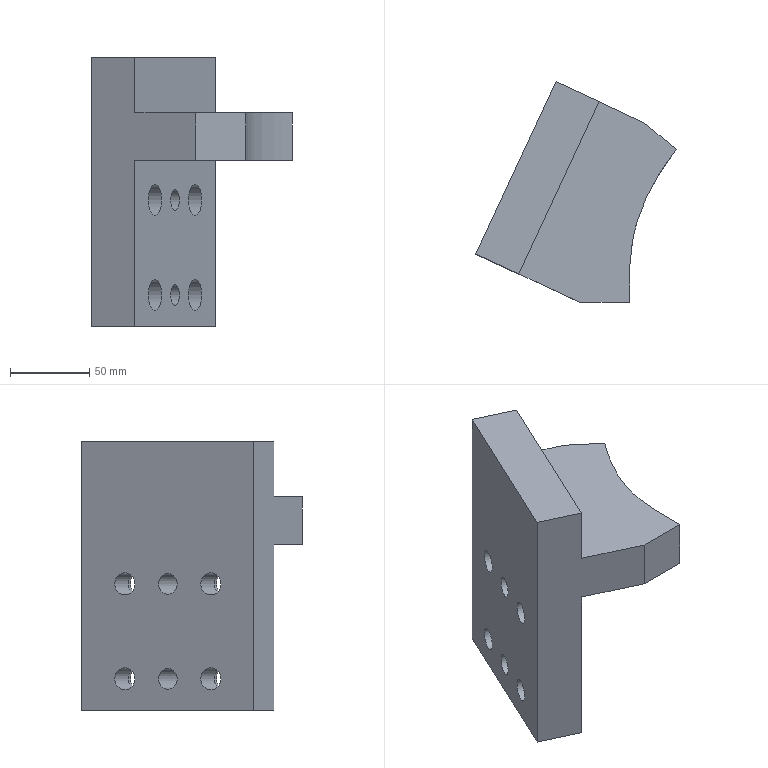Part | NX | features solid 2 | 1 solid | 26 faces | box 126.563 x 139.312 x 170 mm | volume 782387 mm3 | plane 15 | cylinder 10 | spline 1 | commonest cylinder face diameters 14 x4 20 x4 13 x2
STEP:
#1=CARTESIAN_POINT('',(-781.971,-28.997,-85.));
#2=VERTEX_POINT('',#1);
#3=CARTESIAN_POINT('',(-777.745,-19.934,-85.));
#4=DIRECTION('',(-0.9063,0.4226,0.));
#5=DIRECTION('',(-0.4226,-0.9063,0.));
#6=AXIS2_PLACEMENT_3D('',#3,#4,#5);
#7=CIRCLE('',#6,10.);
#8=EDGE_CURVE('',#2,#2,#7,.F.);
#9=ORIENTED_EDGE('',*,*,#8,.F.);
#10=EDGE_LOOP('',(#9));
#11=FACE_BOUND('',#10,.T.);
#12=CARTESIAN_POINT('',(-781.971,-28.997,-25.));
#13=VERTEX_POINT('',#12);
#14=CARTESIAN_POINT('',(-777.745,-19.934,-25.));
#15=DIRECTION('',(-0.9063,0.4226,0.));
#16=DIRECTION('',(-0.4226,-0.9063,0.));
#17=AXIS2_PLACEMENT_3D('',#14,#15,#16);
#18=CIRCLE('',#17,10.);
#19=EDGE_CURVE('',#13,#13,#18,.F.);
#20=ORIENTED_EDGE('',*,*,#19,.F.);
#21=EDGE_LOOP('',(#20));
#22=FACE_BOUND('',#21,.T.);
#23=CARTESIAN_POINT('',(-762.319,13.146,-85.));
#24=VERTEX_POINT('',#23);
#25=CARTESIAN_POINT('',(-765.066,7.255,-85.));
#26=DIRECTION('',(0.9063,-0.4226,0.));
#27=DIRECTION('',(0.4226,0.9063,0.));
#28=AXIS2_PLACEMENT_3D('',#25,#26,#27);
#29=CIRCLE('',#28,6.5);
#30=EDGE_CURVE('',#24,#24,#29,.T.);
#31=ORIENTED_EDGE('',*,*,#30,.F.);
#32=EDGE_LOOP('',(#31));
#33=FACE_BOUND('',#32,.T.);
#34=CARTESIAN_POINT('',(-739.709,61.634,0.));
#35=VERTEX_POINT('',#34);
#36=CARTESIAN_POINT('',(-739.709,61.634,-105.));
#37=VERTEX_POINT('',#36);
#38=CARTESIAN_POINT('',(-739.709,61.634,-162.739));
#39=DIRECTION('',(0.,0.,-1.));
#40=VECTOR('',#39,1000.);
#41=LINE('',#38,#40);
#42=EDGE_CURVE('',#35,#37,#41,.T.);
#43=ORIENTED_EDGE('',*,*,#42,.F.);
#44=CARTESIAN_POINT('',(-790.423,-47.123,0.));
#45=VERTEX_POINT('',#44);
#46=CARTESIAN_POINT('',(-811.528,-92.383,0.));
#47=DIRECTION('',(0.4226,0.9063,0.));
#48=VECTOR('',#47,1000.);
#49=LINE('',#46,#48);
#50=EDGE_CURVE('',#45,#35,#49,.T.);
#51=ORIENTED_EDGE('',*,*,#50,.F.);
#52=CARTESIAN_POINT('',(-790.423,-47.123,-105.));
#53=VERTEX_POINT('',#52);
#54=CARTESIAN_POINT('',(-790.423,-47.123,65.));
#55=DIRECTION('',(0.,0.,1.));
#56=VECTOR('',#55,1000.);
#57=LINE('',#54,#56);
#58=EDGE_CURVE('',#45,#53,#57,.F.);
#59=ORIENTED_EDGE('',*,*,#58,.T.);
#60=CARTESIAN_POINT('',(-811.528,-92.383,-105.));
#61=DIRECTION('',(-0.4226,-0.9063,0.));
#62=VECTOR('',#61,1000.);
#63=LINE('',#60,#62);
#64=EDGE_CURVE('',#53,#37,#63,.F.);
#65=ORIENTED_EDGE('',*,*,#64,.T.);
#66=EDGE_LOOP('',(#43,#51,#59,#65));
#67=FACE_BOUND('',#66,.T.);
#68=CARTESIAN_POINT('',(-762.319,13.146,-25.));
#69=VERTEX_POINT('',#68);
#70=CARTESIAN_POINT('',(-765.066,7.255,-25.));
#71=DIRECTION('',(0.9063,-0.4226,0.));
#72=DIRECTION('',(0.4226,0.9063,0.));
#73=AXIS2_PLACEMENT_3D('',#70,#71,#72);
#74=CIRCLE('',#73,6.5);
#75=EDGE_CURVE('',#69,#69,#74,.T.);
#76=ORIENTED_EDGE('',*,*,#75,.F.);
#77=EDGE_LOOP('',(#76));
#78=FACE_BOUND('',#77,.T.);
#79=CARTESIAN_POINT('',(-756.614,25.381,-25.));
#80=VERTEX_POINT('',#79);
#81=CARTESIAN_POINT('',(-752.388,34.445,-25.));
#82=DIRECTION('',(-0.9063,0.4226,0.));
#83=DIRECTION('',(-0.4226,-0.9063,0.));
#84=AXIS2_PLACEMENT_3D('',#81,#82,#83);
#85=CIRCLE('',#84,10.);
#86=EDGE_CURVE('',#80,#80,#85,.F.);
#87=ORIENTED_EDGE('',*,*,#86,.F.);
#88=EDGE_LOOP('',(#87));
#89=FACE_BOUND('',#88,.T.);
#90=CARTESIAN_POINT('',(-756.614,25.381,-85.));
#91=VERTEX_POINT('',#90);
#92=CARTESIAN_POINT('',(-752.388,34.445,-85.));
#93=DIRECTION('',(-0.9063,0.4226,0.));
#94=DIRECTION('',(-0.4226,-0.9063,0.));
#95=AXIS2_PLACEMENT_3D('',#92,#93,#94);
#96=CIRCLE('',#95,10.);
#97=EDGE_CURVE('',#91,#91,#96,.F.);
#98=ORIENTED_EDGE('',*,*,#97,.F.);
#99=EDGE_LOOP('',(#98));
#100=FACE_BOUND('',#99,.T.);
#101=CARTESIAN_POINT('',(-811.528,-92.383,65.));
#102=DIRECTION('',(-0.9063,0.4226,0.));
#103=DIRECTION('',(-0.4226,-0.9063,0.));
#104=AXIS2_PLACEMENT_3D('',#101,#102,#103);
#105=PLANE('',#104);
#106=ADVANCED_FACE('',(#11,#22,#33,#67,#78,#89,#100),#105,.F.);
#107=CARTESIAN_POINT('',(-789.508,25.825,-85.));
#108=VERTEX_POINT('',#107);
#109=CARTESIAN_POINT('',(-792.255,19.934,-85.));
#110=DIRECTION('',(0.9063,-0.4226,0.));
#111=DIRECTION('',(0.4226,0.9063,0.));
#112=AXIS2_PLACEMENT_3D('',#109,#110,#111);
#113=CIRCLE('',#112,6.5);
#114=EDGE_CURVE('',#108,#108,#113,.T.);
#115=ORIENTED_EDGE('',*,*,#114,.T.);
#116=EDGE_LOOP('',(#115));
#117=FACE_BOUND('',#116,.T.);
#118=CARTESIAN_POINT('',(-776.618,53.467,-25.));
#119=VERTEX_POINT('',#118);
#120=CARTESIAN_POINT('',(-779.577,47.123,-25.));
#121=DIRECTION('',(0.9063,-0.4226,0.));
#122=DIRECTION('',(0.4226,0.9063,0.));
#123=AXIS2_PLACEMENT_3D('',#120,#121,#122);
#124=CIRCLE('',#123,7.);
#125=EDGE_CURVE('',#119,#119,#124,.T.);
#126=ORIENTED_EDGE('',*,*,#125,.T.);
#127=EDGE_LOOP('',(#126));
#128=FACE_BOUND('',#127,.T.);
#129=CARTESIAN_POINT('',(-801.976,-0.9112,-25.));
#130=VERTEX_POINT('',#129);
#131=CARTESIAN_POINT('',(-804.934,-7.255,-25.));
#132=DIRECTION('',(0.9063,-0.4226,0.));
#133=DIRECTION('',(0.4226,0.9063,0.));
#134=AXIS2_PLACEMENT_3D('',#131,#132,#133);
#135=CIRCLE('',#134,7.);
#136=EDGE_CURVE('',#130,#130,#135,.T.);
#137=ORIENTED_EDGE('',*,*,#136,.T.);
#138=EDGE_LOOP('',(#137));
#139=FACE_BOUND('',#138,.T.);
#140=CARTESIAN_POINT('',(-817.612,-34.445,-105.));
#141=VERTEX_POINT('',#140);
#142=CARTESIAN_POINT('',(-766.898,74.312,-105.));
#143=VERTEX_POINT('',#142);
#144=CARTESIAN_POINT('',(-838.718,-79.705,-105.));
#145=DIRECTION('',(-0.4226,-0.9063,0.));
#146=VECTOR('',#145,1000.);
#147=LINE('',#144,#146);
#148=EDGE_CURVE('',#141,#143,#147,.F.);
#149=ORIENTED_EDGE('',*,*,#148,.F.);
#150=CARTESIAN_POINT('',(-817.612,-34.445,65.));
#151=VERTEX_POINT('',#150);
#152=CARTESIAN_POINT('',(-817.612,-34.445,65.));
#153=DIRECTION('',(0.,0.,1.));
#154=VECTOR('',#153,1000.);
#155=LINE('',#152,#154);
#156=EDGE_CURVE('',#151,#141,#155,.F.);
#157=ORIENTED_EDGE('',*,*,#156,.F.);
#158=CARTESIAN_POINT('',(-766.898,74.312,65.));
#159=VERTEX_POINT('',#158);
#160=CARTESIAN_POINT('',(-838.718,-79.705,65.));
#161=DIRECTION('',(0.4226,0.9063,0.));
#162=VECTOR('',#161,1000.);
#163=LINE('',#160,#162);
#164=EDGE_CURVE('',#151,#159,#163,.T.);
#165=ORIENTED_EDGE('',*,*,#164,.T.);
#166=CARTESIAN_POINT('',(-766.898,74.312,-162.739));
#167=DIRECTION('',(0.,0.,-1.));
#168=VECTOR('',#167,1000.);
#169=LINE('',#166,#168);
#170=EDGE_CURVE('',#159,#143,#169,.T.);
#171=ORIENTED_EDGE('',*,*,#170,.T.);
#172=EDGE_LOOP('',(#149,#157,#165,#171));
#173=FACE_BOUND('',#172,.T.);
#174=CARTESIAN_POINT('',(-789.508,25.825,-25.));
#175=VERTEX_POINT('',#174);
#176=CARTESIAN_POINT('',(-792.255,19.934,-25.));
#177=DIRECTION('',(0.9063,-0.4226,0.));
#178=DIRECTION('',(0.4226,0.9063,0.));
#179=AXIS2_PLACEMENT_3D('',#176,#177,#178);
#180=CIRCLE('',#179,6.5);
#181=EDGE_CURVE('',#175,#175,#180,.T.);
#182=ORIENTED_EDGE('',*,*,#181,.T.);
#183=EDGE_LOOP('',(#182));
#184=FACE_BOUND('',#183,.T.);
#185=CARTESIAN_POINT('',(-801.976,-0.9112,-85.));
#186=VERTEX_POINT('',#185);
#187=CARTESIAN_POINT('',(-804.934,-7.255,-85.));
#188=DIRECTION('',(0.9063,-0.4226,0.));
#189=DIRECTION('',(0.4226,0.9063,0.));
#190=AXIS2_PLACEMENT_3D('',#187,#188,#189);
#191=CIRCLE('',#190,7.);
#192=EDGE_CURVE('',#186,#186,#191,.T.);
#193=ORIENTED_EDGE('',*,*,#192,.T.);
#194=EDGE_LOOP('',(#193));
#195=FACE_BOUND('',#194,.T.);
#196=CARTESIAN_POINT('',(-776.618,53.467,-85.));
#197=VERTEX_POINT('',#196);
#198=CARTESIAN_POINT('',(-779.577,47.123,-85.));
#199=DIRECTION('',(0.9063,-0.4226,0.));
#200=DIRECTION('',(0.4226,0.9063,0.));
#201=AXIS2_PLACEMENT_3D('',#198,#199,#200);
#202=CIRCLE('',#201,7.);
#203=EDGE_CURVE('',#197,#197,#202,.T.);
#204=ORIENTED_EDGE('',*,*,#203,.T.);
#205=EDGE_LOOP('',(#204));
#206=FACE_BOUND('',#205,.T.);
#207=CARTESIAN_POINT('',(-838.718,-79.705,65.));
#208=DIRECTION('',(-0.9063,0.4226,0.));
#209=DIRECTION('',(-0.4226,-0.9063,0.));
#210=AXIS2_PLACEMENT_3D('',#207,#208,#209);
#211=PLANE('',#210);
#212=ADVANCED_FACE('',(#117,#128,#139,#173,#184,#195,#206),#211,.T.);
#213=CARTESIAN_POINT('',(-790.423,-47.123,30.));
#214=VERTEX_POINT('',#213);
#215=CARTESIAN_POINT('',(-739.709,61.634,30.));
#216=VERTEX_POINT('',#215);
#217=CARTESIAN_POINT('',(-811.528,-92.383,30.));
#218=DIRECTION('',(0.4226,0.9063,0.));
#219=VECTOR('',#218,1000.);
#220=LINE('',#217,#219);
#221=EDGE_CURVE('',#214,#216,#220,.T.);
#222=ORIENTED_EDGE('',*,*,#221,.T.);
#223=CARTESIAN_POINT('',(-739.709,61.634,65.));
#224=VERTEX_POINT('',#223);
#225=CARTESIAN_POINT('',(-739.709,61.634,-162.739));
#226=DIRECTION('',(0.,0.,-1.));
#227=VECTOR('',#226,1000.);
#228=LINE('',#225,#227);
#229=EDGE_CURVE('',#224,#216,#228,.T.);
#230=ORIENTED_EDGE('',*,*,#229,.F.);
#231=CARTESIAN_POINT('',(-790.423,-47.123,65.));
#232=VERTEX_POINT('',#231);
#233=CARTESIAN_POINT('',(-811.528,-92.383,65.));
#234=DIRECTION('',(0.4226,0.9063,0.));
#235=VECTOR('',#234,1000.);
#236=LINE('',#233,#235);
#237=EDGE_CURVE('',#232,#224,#236,.T.);
#238=ORIENTED_EDGE('',*,*,#237,.F.);
#239=CARTESIAN_POINT('',(-790.423,-47.123,65.));
#240=DIRECTION('',(0.,0.,1.));
#241=VECTOR('',#240,1000.);
#242=LINE('',#239,#241);
#243=EDGE_CURVE('',#232,#214,#242,.F.);
#244=ORIENTED_EDGE('',*,*,#243,.T.);
#245=EDGE_LOOP('',(#222,#230,#238,#244));
#246=FACE_BOUND('',#245,.T.);
#247=CARTESIAN_POINT('',(-811.528,-92.383,65.));
#248=DIRECTION('',(-0.9063,0.4226,0.));
#249=DIRECTION('',(-0.4226,-0.9063,0.));
#250=AXIS2_PLACEMENT_3D('',#247,#248,#249);
#251=PLANE('',#250);
#252=ADVANCED_FACE('',(#246),#251,.F.);
#253=CARTESIAN_POINT('',(-799.486,-42.897,65.));
#254=DIRECTION('',(0.9063,-0.4226,0.));
#255=VECTOR('',#254,1000.);
#256=LINE('',#253,#255);
#257=EDGE_CURVE('',#232,#151,#256,.F.);
#258=ORIENTED_EDGE('',*,*,#257,.F.);
#259=ORIENTED_EDGE('',*,*,#237,.T.);
#260=CARTESIAN_POINT('',(-748.772,65.86,65.));
#261=DIRECTION('',(-0.9063,0.4226,0.));
#262=VECTOR('',#261,1000.);
#263=LINE('',#260,#262);
#264=EDGE_CURVE('',#224,#159,#263,.T.);
#265=ORIENTED_EDGE('',*,*,#264,.T.);
#266=ORIENTED_EDGE('',*,*,#164,.F.);
#267=EDGE_LOOP('',(#258,#259,#265,#266));
#268=FACE_BOUND('',#267,.T.);
#269=CARTESIAN_POINT('',(-820.591,-88.157,65.));
#270=DIRECTION('',(0.,0.,1.));
#271=DIRECTION('',(0.4226,0.9063,0.));
#272=AXIS2_PLACEMENT_3D('',#269,#270,#271);
#273=PLANE('',#272);
#274=ADVANCED_FACE('',(#268),#273,.T.);
#275=CARTESIAN_POINT('',(-710.78,48.144,0.));
#276=VERTEX_POINT('',#275);
#277=CARTESIAN_POINT('',(-710.78,48.144,30.));
#278=VERTEX_POINT('',#277);
#279=CARTESIAN_POINT('',(-710.78,48.144,-162.739));
#280=DIRECTION('',(0.,0.,1.));
#281=VECTOR('',#280,1000.);
#282=LINE('',#279,#281);
#283=EDGE_CURVE('',#276,#278,#282,.T.);
#284=ORIENTED_EDGE('',*,*,#283,.F.);
#285=CARTESIAN_POINT('',(-748.772,65.86,0.));
#286=DIRECTION('',(0.9063,-0.4226,0.));
#287=VECTOR('',#286,1000.);
#288=LINE('',#285,#287);
#289=EDGE_CURVE('',#35,#276,#288,.T.);
#290=ORIENTED_EDGE('',*,*,#289,.F.);
#291=ORIENTED_EDGE('',*,*,#42,.T.);
#292=CARTESIAN_POINT('',(-829.041,103.29,-105.));
#293=DIRECTION('',(0.9063,-0.4226,0.));
#294=VECTOR('',#293,1000.);
#295=LINE('',#292,#294);
#296=EDGE_CURVE('',#37,#143,#295,.F.);
#297=ORIENTED_EDGE('',*,*,#296,.T.);
#298=ORIENTED_EDGE('',*,*,#170,.F.);
#299=ORIENTED_EDGE('',*,*,#264,.F.);
#300=ORIENTED_EDGE('',*,*,#229,.T.);
#301=CARTESIAN_POINT('',(-748.772,65.86,30.));
#302=DIRECTION('',(0.9063,-0.4226,0.));
#303=VECTOR('',#302,1000.);
#304=LINE('',#301,#303);
#305=EDGE_CURVE('',#216,#278,#304,.T.);
#306=ORIENTED_EDGE('',*,*,#305,.T.);
#307=EDGE_LOOP('',(#284,#290,#291,#297,#298,#299,#300,#306));
#308=FACE_BOUND('',#307,.T.);
#309=CARTESIAN_POINT('',(-829.041,103.29,-162.739));
#310=DIRECTION('',(0.4226,0.9063,0.));
#311=DIRECTION('',(0.,0.,-1.));
#312=AXIS2_PLACEMENT_3D('',#309,#310,#311);
#313=PLANE('',#312);
#314=ADVANCED_FACE('',(#308),#313,.T.);
#315=ORIENTED_EDGE('',*,*,#296,.F.);
#316=ORIENTED_EDGE('',*,*,#64,.F.);
#317=CARTESIAN_POINT('',(-879.755,-5.467,-105.));
#318=DIRECTION('',(-0.9063,0.4226,0.));
#319=VECTOR('',#318,1000.);
#320=LINE('',#317,#319);
#321=EDGE_CURVE('',#53,#141,#320,.T.);
#322=ORIENTED_EDGE('',*,*,#321,.T.);
#323=ORIENTED_EDGE('',*,*,#148,.T.);
#324=EDGE_LOOP('',(#315,#316,#322,#323));
#325=FACE_BOUND('',#324,.T.);
#326=CARTESIAN_POINT('',(-820.591,-88.157,-105.));
#327=DIRECTION('',(0.,0.,1.));
#328=DIRECTION('',(0.4226,0.9063,0.));
#329=AXIS2_PLACEMENT_3D('',#326,#327,#328);
#330=PLANE('',#329);
#331=ADVANCED_FACE('',(#325),#330,.F.);
#332=CARTESIAN_POINT('',(-752.086,-65.,30.));
#333=VERTEX_POINT('',#332);
#334=CARTESIAN_POINT('',(-752.086,-65.,0.));
#335=VERTEX_POINT('',#334);
#336=CARTESIAN_POINT('',(-752.086,-65.,-162.739));
#337=DIRECTION('',(0.,0.,1.));
#338=VECTOR('',#337,1000.);
#339=LINE('',#336,#338);
#340=EDGE_CURVE('',#333,#335,#339,.F.);
#341=ORIENTED_EDGE('',*,*,#340,.F.);
#342=CARTESIAN_POINT('',(-879.755,-5.467,30.));
#343=DIRECTION('',(-0.9063,0.4226,0.));
#344=VECTOR('',#343,1000.);
#345=LINE('',#342,#344);
#346=EDGE_CURVE('',#214,#333,#345,.F.);
#347=ORIENTED_EDGE('',*,*,#346,.F.);
#348=ORIENTED_EDGE('',*,*,#243,.F.);
#349=ORIENTED_EDGE('',*,*,#257,.T.);
#350=ORIENTED_EDGE('',*,*,#156,.T.);
#351=ORIENTED_EDGE('',*,*,#321,.F.);
#352=ORIENTED_EDGE('',*,*,#58,.F.);
#353=CARTESIAN_POINT('',(-879.755,-5.467,0.));
#354=DIRECTION('',(-0.9063,0.4226,0.));
#355=VECTOR('',#354,1000.);
#356=LINE('',#353,#355);
#357=EDGE_CURVE('',#45,#335,#356,.F.);
#358=ORIENTED_EDGE('',*,*,#357,.T.);
#359=EDGE_LOOP('',(#341,#347,#348,#349,#350,#351,#352,#358));
#360=FACE_BOUND('',#359,.T.);
#361=CARTESIAN_POINT('',(-879.755,-5.467,-162.739));
#362=DIRECTION('',(0.4226,0.9063,0.));
#363=DIRECTION('',(0.,0.,-1.));
#364=AXIS2_PLACEMENT_3D('',#361,#362,#363);
#365=PLANE('',#364);
#366=ADVANCED_FACE('',(#360),#365,.F.);
#367=CARTESIAN_POINT('',(-691.05,31.588,30.));
#368=VERTEX_POINT('',#367);
#369=CARTESIAN_POINT('',(-691.05,31.588,0.));
#370=VERTEX_POINT('',#369);
#371=CARTESIAN_POINT('',(-691.05,31.588,15.));
#372=DIRECTION('',(0.,0.,1.));
#373=VECTOR('',#372,1000.);
#374=LINE('',#371,#373);
#375=EDGE_CURVE('',#368,#370,#374,.F.);
#376=ORIENTED_EDGE('',*,*,#375,.F.);
#377=CARTESIAN_POINT('',(-720.485,-65.,30.));
#378=VERTEX_POINT('',#377);
#379=CARTESIAN_POINT('',(-720.485,-65.,30.));
#380=CARTESIAN_POINT('',(-720.54,-56.353,30.));
#381=CARTESIAN_POINT('',(-720.797,-43.409,30.));
#382=CARTESIAN_POINT('',(-718.853,-26.087,30.));
#383=CARTESIAN_POINT('',(-715.83,-13.565,30.));
#384=CARTESIAN_POINT('',(-711.315,-1.578,30.));
#385=CARTESIAN_POINT('',(-705.427,10.002,30.));
#386=CARTESIAN_POINT('',(-698.566,21.022,30.));
#387=CARTESIAN_POINT('',(-693.55,28.061,30.));
#388=CARTESIAN_POINT('',(-691.05,31.588,30.));
#389=B_SPLINE_CURVE_WITH_KNOTS('',3,(#379,#380,#381,#382,#383,#384,#385,#386,#387,#388),.UNSPECIFIED.,.F.,.F.,(4,1,1,1,1,1,1,4),(0.01474,0.04067,0.05363,0.0666,0.07956,0.09252,0.1055,0.1185),.UNSPECIFIED.);
#390=EDGE_CURVE('',#378,#368,#389,.T.);
#391=ORIENTED_EDGE('',*,*,#390,.F.);
#392=CARTESIAN_POINT('',(-720.485,-65.,0.));
#393=VERTEX_POINT('',#392);
#394=CARTESIAN_POINT('',(-720.485,-65.,15.));
#395=DIRECTION('',(0.,0.,1.));
#396=VECTOR('',#395,1000.);
#397=LINE('',#394,#396);
#398=EDGE_CURVE('',#393,#378,#397,.T.);
#399=ORIENTED_EDGE('',*,*,#398,.F.);
#400=CARTESIAN_POINT('',(-720.485,-65.,0.));
#401=CARTESIAN_POINT('',(-720.54,-56.331,0.));
#402=CARTESIAN_POINT('',(-720.797,-43.353,0.));
#403=CARTESIAN_POINT('',(-718.841,-26.02,0.));
#404=CARTESIAN_POINT('',(-715.811,-13.506,0.));
#405=CARTESIAN_POINT('',(-711.296,-1.541,0.));
#406=CARTESIAN_POINT('',(-705.434,9.989,0.));
#407=CARTESIAN_POINT('',(-698.562,21.029,0.));
#408=CARTESIAN_POINT('',(-693.549,28.062,0.));
#409=CARTESIAN_POINT('',(-691.05,31.588,0.));
#410=B_SPLINE_CURVE_WITH_KNOTS('',3,(#400,#401,#402,#403,#404,#405,#406,#407,#408,#409),.UNSPECIFIED.,.F.,.F.,(4,1,1,1,1,1,1,4),(0.5103,0.5363,0.5493,0.5623,0.5753,0.5883,0.6013,0.6143),.UNSPECIFIED.);
#411=EDGE_CURVE('',#393,#370,#410,.T.);
#412=ORIENTED_EDGE('',*,*,#411,.T.);
#413=EDGE_LOOP('',(#376,#391,#399,#412));
#414=FACE_BOUND('',#413,.T.);
#415=CARTESIAN_POINT('',(-720.485,-65.,0.));
#416=CARTESIAN_POINT('',(-720.485,-65.,30.));
#417=CARTESIAN_POINT('',(-720.535,-57.144,0.));
#418=CARTESIAN_POINT('',(-720.535,-57.144,30.));
#419=CARTESIAN_POINT('',(-720.799,-44.996,0.));
#420=CARTESIAN_POINT('',(-720.799,-44.996,30.));
#421=CARTESIAN_POINT('',(-719.142,-27.812,0.));
#422=CARTESIAN_POINT('',(-719.142,-27.812,30.));
#423=CARTESIAN_POINT('',(-716.222,-14.711,0.));
#424=CARTESIAN_POINT('',(-716.222,-14.711,30.));
#425=CARTESIAN_POINT('',(-711.385,-1.66,0.));
#426=CARTESIAN_POINT('',(-711.385,-1.66,30.));
#427=CARTESIAN_POINT('',(-705.309,10.218,0.));
#428=CARTESIAN_POINT('',(-705.309,10.218,30.));
#429=CARTESIAN_POINT('',(-699.519,19.467,0.));
#430=CARTESIAN_POINT('',(-699.519,19.467,30.));
#431=CARTESIAN_POINT('',(-694.643,26.543,0.));
#432=CARTESIAN_POINT('',(-694.643,26.543,30.));
#433=CARTESIAN_POINT('',(-692.243,29.905,0.));
#434=CARTESIAN_POINT('',(-692.243,29.905,30.));
#435=CARTESIAN_POINT('',(-691.05,31.588,0.));
#436=CARTESIAN_POINT('',(-691.05,31.588,30.));
#437=B_SPLINE_SURFACE_WITH_KNOTS('',3,1,((#415,#416),(#417,#418),(#419,#420),(#421,#422),(#423,#424),(#425,#426),(#427,#428),(#429,#430),(#431,#432),(#433,#434),(#435,#436)),.SURF_OF_LINEAR_EXTRUSION.,.F.,.F.,.F.,(4,1,1,1,1,1,1,1,4),(2,2),(0.09991,0.3357,0.4536,0.5715,0.6894,0.8073,0.9252,0.9842,1.043),(0.,1.),.UNSPECIFIED.);
#438=ADVANCED_FACE('',(#414),#437,.T.);
#439=CARTESIAN_POINT('',(-708.105,45.899,0.));
#440=DIRECTION('',(-0.766,0.6428,0.));
#441=VECTOR('',#440,1000.);
#442=LINE('',#439,#441);
#443=EDGE_CURVE('',#370,#276,#442,.T.);
#444=ORIENTED_EDGE('',*,*,#443,.F.);
#445=ORIENTED_EDGE('',*,*,#411,.F.);
#446=CARTESIAN_POINT('',(-820.591,-65.,0.));
#447=DIRECTION('',(1.,0.,0.));
#448=VECTOR('',#447,1000.);
#449=LINE('',#446,#448);
#450=EDGE_CURVE('',#335,#393,#449,.T.);
#451=ORIENTED_EDGE('',*,*,#450,.F.);
#452=ORIENTED_EDGE('',*,*,#357,.F.);
#453=ORIENTED_EDGE('',*,*,#50,.T.);
#454=ORIENTED_EDGE('',*,*,#289,.T.);
#455=EDGE_LOOP('',(#444,#445,#451,#452,#453,#454));
#456=FACE_BOUND('',#455,.T.);
#457=CARTESIAN_POINT('',(-820.591,-88.157,0.));
#458=DIRECTION('',(0.,0.,-1.));
#459=DIRECTION('',(-0.9975,0.07067,0.));
#460=AXIS2_PLACEMENT_3D('',#457,#458,#459);
#461=PLANE('',#460);
#462=ADVANCED_FACE('',(#456),#461,.T.);
#463=ORIENTED_EDGE('',*,*,#390,.T.);
#464=CARTESIAN_POINT('',(-708.105,45.899,30.));
#465=DIRECTION('',(-0.766,0.6428,0.));
#466=VECTOR('',#465,1000.);
#467=LINE('',#464,#466);
#468=EDGE_CURVE('',#368,#278,#467,.T.);
#469=ORIENTED_EDGE('',*,*,#468,.T.);
#470=ORIENTED_EDGE('',*,*,#305,.F.);
#471=ORIENTED_EDGE('',*,*,#221,.F.);
#472=ORIENTED_EDGE('',*,*,#346,.T.);
#473=CARTESIAN_POINT('',(-820.591,-65.,30.));
#474=DIRECTION('',(1.,0.,0.));
#475=VECTOR('',#474,1000.);
#476=LINE('',#473,#475);
#477=EDGE_CURVE('',#333,#378,#476,.T.);
#478=ORIENTED_EDGE('',*,*,#477,.T.);
#479=EDGE_LOOP('',(#463,#469,#470,#471,#472,#478));
#480=FACE_BOUND('',#479,.T.);
#481=CARTESIAN_POINT('',(-820.591,-88.157,30.));
#482=DIRECTION('',(0.,0.,-1.));
#483=DIRECTION('',(-0.9975,0.07067,0.));
#484=AXIS2_PLACEMENT_3D('',#481,#482,#483);
#485=PLANE('',#484);
#486=ADVANCED_FACE('',(#480),#485,.F.);
#487=CARTESIAN_POINT('',(-783.849,-9.364,-25.));
#488=VERTEX_POINT('',#487);
#489=CARTESIAN_POINT('',(-786.808,-15.708,-25.));
#490=DIRECTION('',(0.9063,-0.4226,0.));
#491=DIRECTION('',(0.4226,0.9063,0.));
#492=AXIS2_PLACEMENT_3D('',#489,#490,#491);
#493=CIRCLE('',#492,7.);
#494=EDGE_CURVE('',#488,#488,#493,.T.);
#495=ORIENTED_EDGE('',*,*,#494,.T.);
#496=EDGE_LOOP('',(#495));
#497=FACE_BOUND('',#496,.T.);
#498=ORIENTED_EDGE('',*,*,#136,.F.);
#499=EDGE_LOOP('',(#498));
#500=FACE_BOUND('',#499,.T.);
#501=CARTESIAN_POINT('',(-904.628,39.233,-25.));
#502=DIRECTION('',(0.9063,-0.4226,0.));
#503=DIRECTION('',(0.4226,0.9063,0.));
#504=AXIS2_PLACEMENT_3D('',#501,#502,#503);
#505=CYLINDRICAL_SURFACE('',#504,7.);
#506=ADVANCED_FACE('',(#497,#500),#505,.F.);
#507=ORIENTED_EDGE('',*,*,#181,.F.);
#508=EDGE_LOOP('',(#507));
#509=FACE_BOUND('',#508,.T.);
#510=ORIENTED_EDGE('',*,*,#75,.T.);
#511=EDGE_LOOP('',(#510));
#512=FACE_BOUND('',#511,.T.);
#513=CARTESIAN_POINT('',(-891.949,66.422,-25.));
#514=DIRECTION('',(0.9063,-0.4226,0.));
#515=DIRECTION('',(0.4226,0.9063,0.));
#516=AXIS2_PLACEMENT_3D('',#513,#514,#515);
#517=CYLINDRICAL_SURFACE('',#516,6.5);
#518=ADVANCED_FACE('',(#509,#512),#517,.F.);
#519=CARTESIAN_POINT('',(-758.492,45.015,-25.));
#520=VERTEX_POINT('',#519);
#521=CARTESIAN_POINT('',(-761.451,38.671,-25.));
#522=DIRECTION('',(0.9063,-0.4226,0.));
#523=DIRECTION('',(0.4226,0.9063,0.));
#524=AXIS2_PLACEMENT_3D('',#521,#522,#523);
#525=CIRCLE('',#524,7.);
#526=EDGE_CURVE('',#520,#520,#525,.T.);
#527=ORIENTED_EDGE('',*,*,#526,.T.);
#528=EDGE_LOOP('',(#527));
#529=FACE_BOUND('',#528,.T.);
#530=ORIENTED_EDGE('',*,*,#125,.F.);
#531=EDGE_LOOP('',(#530));
#532=FACE_BOUND('',#531,.T.);
#533=CARTESIAN_POINT('',(-879.271,93.611,-25.));
#534=DIRECTION('',(0.9063,-0.4226,0.));
#535=DIRECTION('',(0.4226,0.9063,0.));
#536=AXIS2_PLACEMENT_3D('',#533,#534,#535);
#537=CYLINDRICAL_SURFACE('',#536,7.);
#538=ADVANCED_FACE('',(#529,#532),#537,.F.);
#539=CARTESIAN_POINT('',(-783.849,-9.364,-85.));
#540=VERTEX_POINT('',#539);
#541=CARTESIAN_POINT('',(-786.808,-15.708,-85.));
#542=DIRECTION('',(0.9063,-0.4226,0.));
#543=DIRECTION('',(0.4226,0.9063,0.));
#544=AXIS2_PLACEMENT_3D('',#541,#542,#543);
#545=CIRCLE('',#544,7.);
#546=EDGE_CURVE('',#540,#540,#545,.T.);
#547=ORIENTED_EDGE('',*,*,#546,.T.);
#548=EDGE_LOOP('',(#547));
#549=FACE_BOUND('',#548,.T.);
#550=ORIENTED_EDGE('',*,*,#192,.F.);
#551=EDGE_LOOP('',(#550));
#552=FACE_BOUND('',#551,.T.);
#553=CARTESIAN_POINT('',(-904.628,39.233,-85.));
#554=DIRECTION('',(0.9063,-0.4226,0.));
#555=DIRECTION('',(0.4226,0.9063,0.));
#556=AXIS2_PLACEMENT_3D('',#553,#554,#555);
#557=CYLINDRICAL_SURFACE('',#556,7.);
#558=ADVANCED_FACE('',(#549,#552),#557,.F.);
#559=ORIENTED_EDGE('',*,*,#114,.F.);
#560=EDGE_LOOP('',(#559));
#561=FACE_BOUND('',#560,.T.);
#562=ORIENTED_EDGE('',*,*,#30,.T.);
#563=EDGE_LOOP('',(#562));
#564=FACE_BOUND('',#563,.T.);
#565=CARTESIAN_POINT('',(-891.949,66.422,-85.));
#566=DIRECTION('',(0.9063,-0.4226,0.));
#567=DIRECTION('',(0.4226,0.9063,0.));
#568=AXIS2_PLACEMENT_3D('',#565,#566,#567);
#569=CYLINDRICAL_SURFACE('',#568,6.5);
#570=ADVANCED_FACE('',(#561,#564),#569,.F.);
#571=CARTESIAN_POINT('',(-758.492,45.015,-85.));
#572=VERTEX_POINT('',#571);
#573=CARTESIAN_POINT('',(-761.451,38.671,-85.));
#574=DIRECTION('',(0.9063,-0.4226,0.));
#575=DIRECTION('',(0.4226,0.9063,0.));
#576=AXIS2_PLACEMENT_3D('',#573,#574,#575);
#577=CIRCLE('',#576,7.);
#578=EDGE_CURVE('',#572,#572,#577,.T.);
#579=ORIENTED_EDGE('',*,*,#578,.T.);
#580=EDGE_LOOP('',(#579));
#581=FACE_BOUND('',#580,.T.);
#582=ORIENTED_EDGE('',*,*,#203,.F.);
#583=EDGE_LOOP('',(#582));
#584=FACE_BOUND('',#583,.T.);
#585=CARTESIAN_POINT('',(-879.271,93.611,-85.));
#586=DIRECTION('',(0.9063,-0.4226,0.));
#587=DIRECTION('',(0.4226,0.9063,0.));
#588=AXIS2_PLACEMENT_3D('',#585,#586,#587);
#589=CYLINDRICAL_SURFACE('',#588,7.);
#590=ADVANCED_FACE('',(#581,#584),#589,.F.);
#591=ORIENTED_EDGE('',*,*,#450,.T.);
#592=ORIENTED_EDGE('',*,*,#398,.T.);
#593=ORIENTED_EDGE('',*,*,#477,.F.);
#594=ORIENTED_EDGE('',*,*,#340,.T.);
#595=EDGE_LOOP('',(#591,#592,#593,#594));
#596=FACE_BOUND('',#595,.T.);
#597=CARTESIAN_POINT('',(-775.,-65.,-35.));
#598=DIRECTION('',(0.,1.,0.));
#599=DIRECTION('',(-1.,0.,0.));
#600=AXIS2_PLACEMENT_3D('',#597,#598,#599);
#601=PLANE('',#600);
#602=ADVANCED_FACE('',(#596),#601,.F.);
#603=ORIENTED_EDGE('',*,*,#443,.T.);
#604=ORIENTED_EDGE('',*,*,#283,.T.);
#605=ORIENTED_EDGE('',*,*,#468,.F.);
#606=ORIENTED_EDGE('',*,*,#375,.T.);
#607=EDGE_LOOP('',(#603,#604,#605,#606));
#608=FACE_BOUND('',#607,.T.);
#609=CARTESIAN_POINT('',(-723.852,59.113,-48.91));
#610=DIRECTION('',(-0.6428,-0.766,0.));
#611=DIRECTION('',(0.766,-0.6428,0.));
#612=AXIS2_PLACEMENT_3D('',#609,#610,#611);
#613=PLANE('',#612);
#614=ADVANCED_FACE('',(#608),#613,.F.);
#615=CARTESIAN_POINT('',(-791.034,-24.771,-25.));
#616=VERTEX_POINT('',#615);
#617=CARTESIAN_POINT('',(-786.808,-15.708,-25.));
#618=DIRECTION('',(-0.9063,0.4226,0.));
#619=DIRECTION('',(-0.4226,-0.9063,0.));
#620=AXIS2_PLACEMENT_3D('',#617,#618,#619);
#621=CIRCLE('',#620,10.);
#622=EDGE_CURVE('',#616,#616,#621,.F.);
#623=ORIENTED_EDGE('',*,*,#622,.F.);
#624=EDGE_LOOP('',(#623));
#625=FACE_BOUND('',#624,.T.);
#626=ORIENTED_EDGE('',*,*,#19,.T.);
#627=EDGE_LOOP('',(#626));
#628=FACE_BOUND('',#627,.T.);
#629=CARTESIAN_POINT('',(-777.745,-19.934,-25.));
#630=DIRECTION('',(-0.9063,0.4226,0.));
#631=DIRECTION('',(-0.4226,-0.9063,0.));
#632=AXIS2_PLACEMENT_3D('',#629,#630,#631);
#633=CYLINDRICAL_SURFACE('',#632,10.);
#634=ADVANCED_FACE('',(#625,#628),#633,.F.);
#635=ORIENTED_EDGE('',*,*,#622,.T.);
#636=EDGE_LOOP('',(#635));
#637=FACE_BOUND('',#636,.T.);
#638=ORIENTED_EDGE('',*,*,#494,.F.);
#639=EDGE_LOOP('',(#638));
#640=FACE_BOUND('',#639,.T.);
#641=CARTESIAN_POINT('',(-786.808,-15.708,-25.));
#642=DIRECTION('',(-0.9063,0.4226,0.));
#643=DIRECTION('',(-0.4226,-0.9063,0.));
#644=AXIS2_PLACEMENT_3D('',#641,#642,#643);
#645=PLANE('',#644);
#646=ADVANCED_FACE('',(#637,#640),#645,.F.);
#647=CARTESIAN_POINT('',(-765.677,29.608,-25.));
#648=VERTEX_POINT('',#647);
#649=CARTESIAN_POINT('',(-761.451,38.671,-25.));
#650=DIRECTION('',(-0.9063,0.4226,0.));
#651=DIRECTION('',(-0.4226,-0.9063,0.));
#652=AXIS2_PLACEMENT_3D('',#649,#650,#651);
#653=CIRCLE('',#652,10.);
#654=EDGE_CURVE('',#648,#648,#653,.F.);
#655=ORIENTED_EDGE('',*,*,#654,.F.);
#656=EDGE_LOOP('',(#655));
#657=FACE_BOUND('',#656,.T.);
#658=ORIENTED_EDGE('',*,*,#86,.T.);
#659=EDGE_LOOP('',(#658));
#660=FACE_BOUND('',#659,.T.);
#661=CARTESIAN_POINT('',(-752.388,34.445,-25.));
#662=DIRECTION('',(-0.9063,0.4226,0.));
#663=DIRECTION('',(-0.4226,-0.9063,0.));
#664=AXIS2_PLACEMENT_3D('',#661,#662,#663);
#665=CYLINDRICAL_SURFACE('',#664,10.);
#666=ADVANCED_FACE('',(#657,#660),#665,.F.);
#667=ORIENTED_EDGE('',*,*,#654,.T.);
#668=EDGE_LOOP('',(#667));
#669=FACE_BOUND('',#668,.T.);
#670=ORIENTED_EDGE('',*,*,#526,.F.);
#671=EDGE_LOOP('',(#670));
#672=FACE_BOUND('',#671,.T.);
#673=CARTESIAN_POINT('',(-761.451,38.671,-25.));
#674=DIRECTION('',(-0.9063,0.4226,0.));
#675=DIRECTION('',(-0.4226,-0.9063,0.));
#676=AXIS2_PLACEMENT_3D('',#673,#674,#675);
#677=PLANE('',#676);
#678=ADVANCED_FACE('',(#669,#672),#677,.F.);
#679=CARTESIAN_POINT('',(-791.034,-24.771,-85.));
#680=VERTEX_POINT('',#679);
#681=CARTESIAN_POINT('',(-786.808,-15.708,-85.));
#682=DIRECTION('',(-0.9063,0.4226,0.));
#683=DIRECTION('',(-0.4226,-0.9063,0.));
#684=AXIS2_PLACEMENT_3D('',#681,#682,#683);
#685=CIRCLE('',#684,10.);
#686=EDGE_CURVE('',#680,#680,#685,.F.);
#687=ORIENTED_EDGE('',*,*,#686,.F.);
#688=EDGE_LOOP('',(#687));
#689=FACE_BOUND('',#688,.T.);
#690=ORIENTED_EDGE('',*,*,#8,.T.);
#691=EDGE_LOOP('',(#690));
#692=FACE_BOUND('',#691,.T.);
#693=CARTESIAN_POINT('',(-777.745,-19.934,-85.));
#694=DIRECTION('',(-0.9063,0.4226,0.));
#695=DIRECTION('',(-0.4226,-0.9063,0.));
#696=AXIS2_PLACEMENT_3D('',#693,#694,#695);
#697=CYLINDRICAL_SURFACE('',#696,10.);
#698=ADVANCED_FACE('',(#689,#692),#697,.F.);
#699=ORIENTED_EDGE('',*,*,#686,.T.);
#700=EDGE_LOOP('',(#699));
#701=FACE_BOUND('',#700,.T.);
#702=ORIENTED_EDGE('',*,*,#546,.F.);
#703=EDGE_LOOP('',(#702));
#704=FACE_BOUND('',#703,.T.);
#705=CARTESIAN_POINT('',(-786.808,-15.708,-85.));
#706=DIRECTION('',(-0.9063,0.4226,0.));
#707=DIRECTION('',(-0.4226,-0.9063,0.));
#708=AXIS2_PLACEMENT_3D('',#705,#706,#707);
#709=PLANE('',#708);
#710=ADVANCED_FACE('',(#701,#704),#709,.F.);
#711=CARTESIAN_POINT('',(-765.677,29.608,-85.));
#712=VERTEX_POINT('',#711);
#713=CARTESIAN_POINT('',(-761.451,38.671,-85.));
#714=DIRECTION('',(-0.9063,0.4226,0.));
#715=DIRECTION('',(-0.4226,-0.9063,0.));
#716=AXIS2_PLACEMENT_3D('',#713,#714,#715);
#717=CIRCLE('',#716,10.);
#718=EDGE_CURVE('',#712,#712,#717,.F.);
#719=ORIENTED_EDGE('',*,*,#718,.F.);
#720=EDGE_LOOP('',(#719));
#721=FACE_BOUND('',#720,.T.);
#722=ORIENTED_EDGE('',*,*,#97,.T.);
#723=EDGE_LOOP('',(#722));
#724=FACE_BOUND('',#723,.T.);
#725=CARTESIAN_POINT('',(-752.388,34.445,-85.));
#726=DIRECTION('',(-0.9063,0.4226,0.));
#727=DIRECTION('',(-0.4226,-0.9063,0.));
#728=AXIS2_PLACEMENT_3D('',#725,#726,#727);
#729=CYLINDRICAL_SURFACE('',#728,10.);
#730=ADVANCED_FACE('',(#721,#724),#729,.F.);
#731=ORIENTED_EDGE('',*,*,#718,.T.);
#732=EDGE_LOOP('',(#731));
#733=FACE_BOUND('',#732,.T.);
#734=ORIENTED_EDGE('',*,*,#578,.F.);
#735=EDGE_LOOP('',(#734));
#736=FACE_BOUND('',#735,.T.);
#737=CARTESIAN_POINT('',(-761.451,38.671,-85.));
#738=DIRECTION('',(-0.9063,0.4226,0.));
#739=DIRECTION('',(-0.4226,-0.9063,0.));
#740=AXIS2_PLACEMENT_3D('',#737,#738,#739);
#741=PLANE('',#740);
#742=ADVANCED_FACE('',(#733,#736),#741,.F.);
#743=CLOSED_SHELL('',(#106,#212,#252,#274,#314,#331,#366,#438,#462,#486,#506,#518,#538,#558,#570,#590,#602,#614,#634,#646,#666,#678,#698,#710,#730,#742));
#744=MANIFOLD_SOLID_BREP('',#743);
#745=(LENGTH_UNIT()NAMED_UNIT(*)SI_UNIT(.MILLI.,.METRE.));
#746=UNCERTAINTY_MEASURE_WITH_UNIT(LENGTH_MEASURE(0.0508),#745,'','');
#747=(NAMED_UNIT(*)PLANE_ANGLE_UNIT()SI_UNIT($,.RADIAN.));
#748=(NAMED_UNIT(*)SI_UNIT($,.STERADIAN.)SOLID_ANGLE_UNIT());
#749=(GEOMETRIC_REPRESENTATION_CONTEXT(3)GLOBAL_UNCERTAINTY_ASSIGNED_CONTEXT((#746))GLOBAL_UNIT_ASSIGNED_CONTEXT((#745,#747,#748))REPRESENTATION_CONTEXT('',''));
#750=ADVANCED_BREP_SHAPE_REPRESENTATION('',(#744),#749);